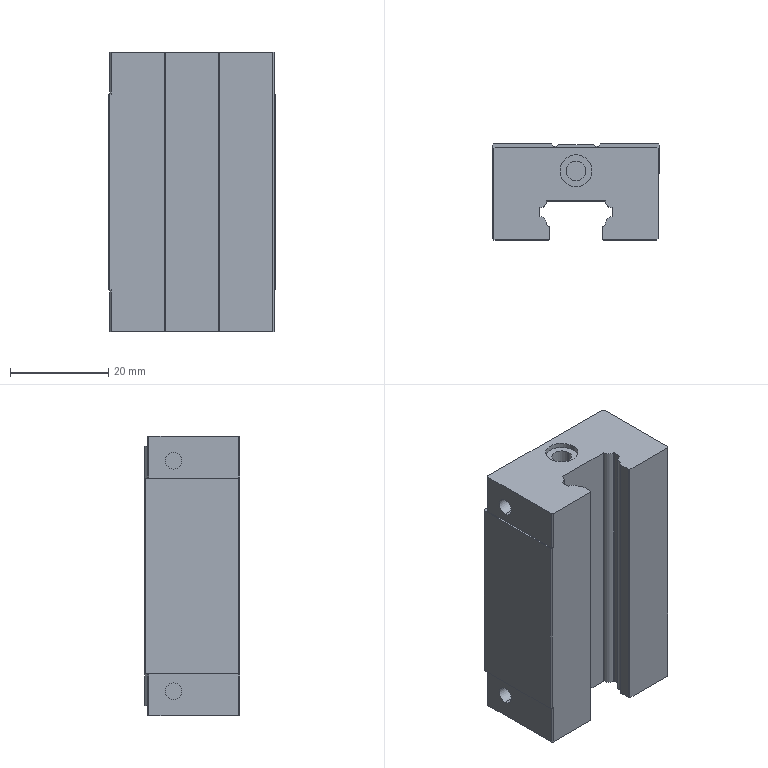Part | SolidWorks | features BaseBody 1 | 1 solid | 211 faces | box 34 x 19.5 x 56.8 mm | volume 30476 mm3 | plane 134 | cylinder 49 | spline 28 | commonest cylinder face diameters 4 x12 0.46 x8 3.35 x8 3 x5 0.74 x4 1 x4